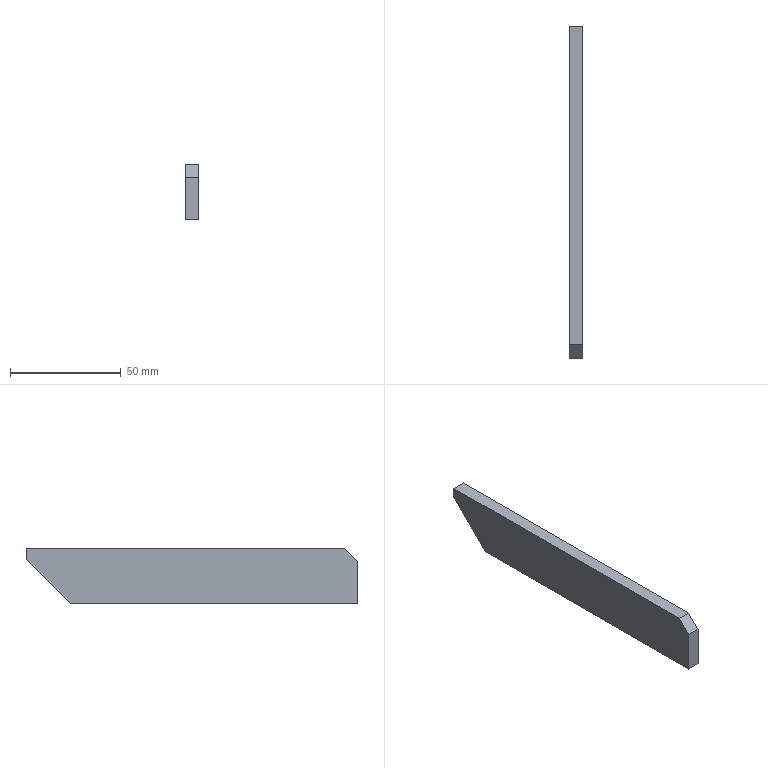Part | NX | 1 solid | 8 faces | box 6 x 150 x 25 mm | volume 21192 mm3 | plane 8
STEP:
#1=CARTESIAN_POINT('',(-147.75,-100.5,-626.4));
#2=VERTEX_POINT('',#1);
#3=CARTESIAN_POINT('',(-147.75,-100.5,-607.4));
#4=VERTEX_POINT('',#3);
#5=CARTESIAN_POINT('',(-147.75,-100.5,-577.5));
#6=DIRECTION('',(0.,0.,1.));
#7=VECTOR('',#6,1000.);
#8=LINE('',#5,#7);
#9=EDGE_CURVE('',#2,#4,#8,.T.);
#10=ORIENTED_EDGE('',*,*,#9,.T.);
#11=CARTESIAN_POINT('',(-147.75,-94.5,-601.4));
#12=VERTEX_POINT('',#11);
#13=CARTESIAN_POINT('',(-147.75,-100.5,-607.4));
#14=DIRECTION('',(0.,-0.7071,-0.7071));
#15=VECTOR('',#14,1000.);
#16=LINE('',#13,#15);
#17=EDGE_CURVE('',#12,#4,#16,.T.);
#18=ORIENTED_EDGE('',*,*,#17,.F.);
#19=CARTESIAN_POINT('',(-147.75,49.5,-601.4));
#20=VERTEX_POINT('',#19);
#21=CARTESIAN_POINT('',(-147.75,-100.5,-601.4));
#22=DIRECTION('',(0.,1.,0.));
#23=VECTOR('',#22,1000.);
#24=LINE('',#21,#23);
#25=EDGE_CURVE('',#12,#20,#24,.T.);
#26=ORIENTED_EDGE('',*,*,#25,.T.);
#27=CARTESIAN_POINT('',(-147.75,49.5,-606.4));
#28=VERTEX_POINT('',#27);
#29=CARTESIAN_POINT('',(-147.75,49.5,-577.5));
#30=DIRECTION('',(0.,0.,1.));
#31=VECTOR('',#30,1000.);
#32=LINE('',#29,#31);
#33=EDGE_CURVE('',#28,#20,#32,.T.);
#34=ORIENTED_EDGE('',*,*,#33,.F.);
#35=CARTESIAN_POINT('',(-147.75,29.5,-626.4));
#36=VERTEX_POINT('',#35);
#37=CARTESIAN_POINT('',(-147.75,-100.5,-756.4));
#38=DIRECTION('',(0.,0.7071,0.7071));
#39=VECTOR('',#38,1000.);
#40=LINE('',#37,#39);
#41=EDGE_CURVE('',#36,#28,#40,.T.);
#42=ORIENTED_EDGE('',*,*,#41,.F.);
#43=CARTESIAN_POINT('',(-147.75,-100.5,-626.4));
#44=DIRECTION('',(0.,1.,0.));
#45=VECTOR('',#44,1000.);
#46=LINE('',#43,#45);
#47=EDGE_CURVE('',#2,#36,#46,.T.);
#48=ORIENTED_EDGE('',*,*,#47,.F.);
#49=EDGE_LOOP('',(#10,#18,#26,#34,#42,#48));
#50=FACE_BOUND('',#49,.T.);
#51=CARTESIAN_POINT('',(-147.75,-100.5,-601.4));
#52=DIRECTION('',(-1.,0.,0.));
#53=DIRECTION('',(0.,0.,1.));
#54=AXIS2_PLACEMENT_3D('',#51,#52,#53);
#55=PLANE('',#54);
#56=ADVANCED_FACE('',(#50),#55,.T.);
#57=CARTESIAN_POINT('',(-141.75,-94.5,-601.4));
#58=VERTEX_POINT('',#57);
#59=CARTESIAN_POINT('',(-161.337,-94.5,-601.4));
#60=DIRECTION('',(-1.,0.,0.));
#61=VECTOR('',#60,1000.);
#62=LINE('',#59,#61);
#63=EDGE_CURVE('',#58,#12,#62,.T.);
#64=ORIENTED_EDGE('',*,*,#63,.F.);
#65=CARTESIAN_POINT('',(-141.75,49.5,-601.4));
#66=VERTEX_POINT('',#65);
#67=CARTESIAN_POINT('',(-141.75,-100.5,-601.4));
#68=DIRECTION('',(0.,1.,0.));
#69=VECTOR('',#68,1000.);
#70=LINE('',#67,#69);
#71=EDGE_CURVE('',#58,#66,#70,.T.);
#72=ORIENTED_EDGE('',*,*,#71,.T.);
#73=CARTESIAN_POINT('',(-144.75,49.5,-601.4));
#74=DIRECTION('',(-1.,0.,0.));
#75=VECTOR('',#74,1000.);
#76=LINE('',#73,#75);
#77=EDGE_CURVE('',#66,#20,#76,.T.);
#78=ORIENTED_EDGE('',*,*,#77,.T.);
#79=ORIENTED_EDGE('',*,*,#25,.F.);
#80=EDGE_LOOP('',(#64,#72,#78,#79));
#81=FACE_BOUND('',#80,.T.);
#82=CARTESIAN_POINT('',(-141.75,-100.5,-601.4));
#83=DIRECTION('',(0.,0.,1.));
#84=DIRECTION('',(1.,0.,0.));
#85=AXIS2_PLACEMENT_3D('',#82,#83,#84);
#86=PLANE('',#85);
#87=ADVANCED_FACE('',(#81),#86,.T.);
#88=CARTESIAN_POINT('',(-141.75,-100.5,-626.4));
#89=VERTEX_POINT('',#88);
#90=CARTESIAN_POINT('',(-141.75,-100.5,-607.4));
#91=VERTEX_POINT('',#90);
#92=CARTESIAN_POINT('',(-141.75,-100.5,-577.5));
#93=DIRECTION('',(0.,0.,1.));
#94=VECTOR('',#93,1000.);
#95=LINE('',#92,#94);
#96=EDGE_CURVE('',#89,#91,#95,.T.);
#97=ORIENTED_EDGE('',*,*,#96,.F.);
#98=CARTESIAN_POINT('',(-141.75,29.5,-626.4));
#99=VERTEX_POINT('',#98);
#100=CARTESIAN_POINT('',(-141.75,-100.5,-626.4));
#101=DIRECTION('',(0.,1.,0.));
#102=VECTOR('',#101,1000.);
#103=LINE('',#100,#102);
#104=EDGE_CURVE('',#89,#99,#103,.T.);
#105=ORIENTED_EDGE('',*,*,#104,.T.);
#106=CARTESIAN_POINT('',(-141.75,49.5,-606.4));
#107=VERTEX_POINT('',#106);
#108=CARTESIAN_POINT('',(-141.75,-100.5,-756.4));
#109=DIRECTION('',(0.,-0.7071,-0.7071));
#110=VECTOR('',#109,1000.);
#111=LINE('',#108,#110);
#112=EDGE_CURVE('',#107,#99,#111,.T.);
#113=ORIENTED_EDGE('',*,*,#112,.F.);
#114=CARTESIAN_POINT('',(-141.75,49.5,-577.5));
#115=DIRECTION('',(0.,0.,1.));
#116=VECTOR('',#115,1000.);
#117=LINE('',#114,#116);
#118=EDGE_CURVE('',#107,#66,#117,.T.);
#119=ORIENTED_EDGE('',*,*,#118,.T.);
#120=ORIENTED_EDGE('',*,*,#71,.F.);
#121=CARTESIAN_POINT('',(-141.75,-100.5,-607.4));
#122=DIRECTION('',(0.,0.7071,0.7071));
#123=VECTOR('',#122,1000.);
#124=LINE('',#121,#123);
#125=EDGE_CURVE('',#91,#58,#124,.T.);
#126=ORIENTED_EDGE('',*,*,#125,.F.);
#127=EDGE_LOOP('',(#97,#105,#113,#119,#120,#126));
#128=FACE_BOUND('',#127,.T.);
#129=CARTESIAN_POINT('',(-141.75,-100.5,-626.4));
#130=DIRECTION('',(1.,0.,0.));
#131=DIRECTION('',(0.,1.,0.));
#132=AXIS2_PLACEMENT_3D('',#129,#130,#131);
#133=PLANE('',#132);
#134=ADVANCED_FACE('',(#128),#133,.T.);
#135=CARTESIAN_POINT('',(-14.5,-100.5,-626.4));
#136=DIRECTION('',(-1.,0.,0.));
#137=VECTOR('',#136,1000.);
#138=LINE('',#135,#137);
#139=EDGE_CURVE('',#89,#2,#138,.T.);
#140=ORIENTED_EDGE('',*,*,#139,.T.);
#141=ORIENTED_EDGE('',*,*,#47,.T.);
#142=CARTESIAN_POINT('',(-161.337,29.5,-626.4));
#143=DIRECTION('',(-1.,0.,0.));
#144=VECTOR('',#143,1000.);
#145=LINE('',#142,#144);
#146=EDGE_CURVE('',#99,#36,#145,.T.);
#147=ORIENTED_EDGE('',*,*,#146,.F.);
#148=ORIENTED_EDGE('',*,*,#104,.F.);
#149=EDGE_LOOP('',(#140,#141,#147,#148));
#150=FACE_BOUND('',#149,.T.);
#151=CARTESIAN_POINT('',(-147.75,-100.5,-626.4));
#152=DIRECTION('',(0.,0.,-1.));
#153=DIRECTION('',(0.,-1.,0.));
#154=AXIS2_PLACEMENT_3D('',#151,#152,#153);
#155=PLANE('',#154);
#156=ADVANCED_FACE('',(#150),#155,.T.);
#157=CARTESIAN_POINT('',(-161.337,49.5,-606.4));
#158=DIRECTION('',(1.,0.,0.));
#159=VECTOR('',#158,1000.);
#160=LINE('',#157,#159);
#161=EDGE_CURVE('',#28,#107,#160,.T.);
#162=ORIENTED_EDGE('',*,*,#161,.F.);
#163=ORIENTED_EDGE('',*,*,#33,.T.);
#164=ORIENTED_EDGE('',*,*,#77,.F.);
#165=ORIENTED_EDGE('',*,*,#118,.F.);
#166=EDGE_LOOP('',(#162,#163,#164,#165));
#167=FACE_BOUND('',#166,.T.);
#168=CARTESIAN_POINT('',(-161.337,49.5,-601.43));
#169=DIRECTION('',(0.,1.,0.));
#170=DIRECTION('',(1.,0.,0.));
#171=AXIS2_PLACEMENT_3D('',#168,#169,#170);
#172=PLANE('',#171);
#173=ADVANCED_FACE('',(#167),#172,.T.);
#174=ORIENTED_EDGE('',*,*,#161,.T.);
#175=ORIENTED_EDGE('',*,*,#112,.T.);
#176=ORIENTED_EDGE('',*,*,#146,.T.);
#177=ORIENTED_EDGE('',*,*,#41,.T.);
#178=EDGE_LOOP('',(#174,#175,#176,#177));
#179=FACE_BOUND('',#178,.T.);
#180=CARTESIAN_POINT('',(-144.75,39.5,-616.4));
#181=DIRECTION('',(0.,0.7071,-0.7071));
#182=DIRECTION('',(-1.,0.,0.));
#183=AXIS2_PLACEMENT_3D('',#180,#181,#182);
#184=PLANE('',#183);
#185=ADVANCED_FACE('',(#179),#184,.T.);
#186=CARTESIAN_POINT('',(-161.337,-100.5,-607.4));
#187=DIRECTION('',(-1.,0.,0.));
#188=VECTOR('',#187,1000.);
#189=LINE('',#186,#188);
#190=EDGE_CURVE('',#91,#4,#189,.T.);
#191=ORIENTED_EDGE('',*,*,#190,.T.);
#192=ORIENTED_EDGE('',*,*,#9,.F.);
#193=ORIENTED_EDGE('',*,*,#139,.F.);
#194=ORIENTED_EDGE('',*,*,#96,.T.);
#195=EDGE_LOOP('',(#191,#192,#193,#194));
#196=FACE_BOUND('',#195,.T.);
#197=CARTESIAN_POINT('',(-161.337,-100.5,-601.43));
#198=DIRECTION('',(0.,1.,0.));
#199=DIRECTION('',(1.,0.,0.));
#200=AXIS2_PLACEMENT_3D('',#197,#198,#199);
#201=PLANE('',#200);
#202=ADVANCED_FACE('',(#196),#201,.F.);
#203=ORIENTED_EDGE('',*,*,#190,.F.);
#204=ORIENTED_EDGE('',*,*,#125,.T.);
#205=ORIENTED_EDGE('',*,*,#63,.T.);
#206=ORIENTED_EDGE('',*,*,#17,.T.);
#207=EDGE_LOOP('',(#203,#204,#205,#206));
#208=FACE_BOUND('',#207,.T.);
#209=CARTESIAN_POINT('',(-144.75,-97.5,-604.4));
#210=DIRECTION('',(0.,-0.7071,0.7071));
#211=DIRECTION('',(-1.,0.,0.));
#212=AXIS2_PLACEMENT_3D('',#209,#210,#211);
#213=PLANE('',#212);
#214=ADVANCED_FACE('',(#208),#213,.T.);
#215=CLOSED_SHELL('',(#56,#87,#134,#156,#173,#185,#202,#214));
#216=MANIFOLD_SOLID_BREP('',#215);
#217=(LENGTH_UNIT()NAMED_UNIT(*)SI_UNIT(.MILLI.,.METRE.));
#218=UNCERTAINTY_MEASURE_WITH_UNIT(LENGTH_MEASURE(0.00001),#217,'','');
#219=(NAMED_UNIT(*)PLANE_ANGLE_UNIT()SI_UNIT($,.RADIAN.));
#220=(NAMED_UNIT(*)SI_UNIT($,.STERADIAN.)SOLID_ANGLE_UNIT());
#221=(GEOMETRIC_REPRESENTATION_CONTEXT(3)GLOBAL_UNCERTAINTY_ASSIGNED_CONTEXT((#218))GLOBAL_UNIT_ASSIGNED_CONTEXT((#217,#219,#220))REPRESENTATION_CONTEXT('',''));
#222=ADVANCED_BREP_SHAPE_REPRESENTATION('',(#216),#221);